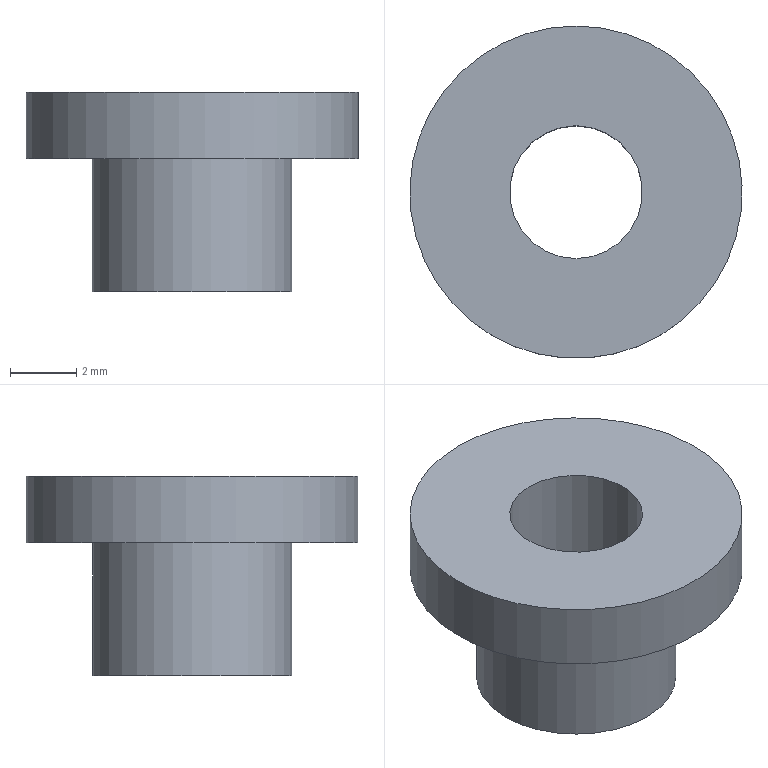Part | STEP file | 1-73.4 | 1 solid | 6 faces | box 10 x 10 x 6 mm | volume 194.779 mm3 | plane 3 | cylinder 3 | commonest cylinder face diameters 4 x1 6 x1 10 x1
STEP:
#1=CARTESIAN_POINT('',(0.,0.,0.));
#2=DIRECTION('',(0.,0.,1.));
#3=DIRECTION('',(1.,0.,0.));
#4=AXIS2_PLACEMENT_3D('',#1,#2,#3);
#5=CARTESIAN_POINT('',(0.,5.,2.));
#6=VERTEX_POINT('',#5);
#7=CARTESIAN_POINT('',(0.,0.,2.));
#8=DIRECTION('',(0.,0.,1.));
#9=DIRECTION('',(0.,1.,0.));
#10=AXIS2_PLACEMENT_3D('',#7,#8,#9);
#11=CIRCLE('',#10,5.);
#12=CARTESIAN_POINT('',(0.,-1.34,2.));
#13=DIRECTION('',(0.,0.,1.));
#14=DIRECTION('',(1.,0.,0.));
#15=AXIS2_PLACEMENT_3D('',#12,#13,#14);
#16=PLANE('',#15);
#17=CARTESIAN_POINT('',(0.,1.34));
#18=DIRECTION('',(0.,1.));
#19=AXIS2_PLACEMENT_2D('',#17,#18);
#20=CIRCLE('',#19,5.);
#21=(GEOMETRIC_REPRESENTATION_CONTEXT(2)PARAMETRIC_REPRESENTATION_CONTEXT()REPRESENTATION_CONTEXT('',''));
#22=DEFINITIONAL_REPRESENTATION('',(#20),#21);
#23=PCURVE('',#16,#22);
#24=CARTESIAN_POINT('',(0.,0.,0.));
#25=DIRECTION('',(0.,0.,1.));
#26=DIRECTION('',(0.,1.,0.));
#27=AXIS2_PLACEMENT_3D('',#24,#25,#26);
#28=CYLINDRICAL_SURFACE('',#27,5.);
#29=CARTESIAN_POINT('',(0.,2.));
#30=DIRECTION('',(1.,0.));
#31=VECTOR('',#30,1.);
#32=LINE('',#29,#31);
#33=(GEOMETRIC_REPRESENTATION_CONTEXT(2)PARAMETRIC_REPRESENTATION_CONTEXT()REPRESENTATION_CONTEXT('',''));
#34=DEFINITIONAL_REPRESENTATION('',(#32),#33);
#35=PCURVE('',#28,#34);
#36=SURFACE_CURVE('',#11,(#23,#35),.PCURVE_S1.);
#37=EDGE_CURVE('',#6,#6,#36,.T.);
#38=ORIENTED_EDGE('',*,*,#37,.T.);
#39=EDGE_LOOP('',(#38));
#40=FACE_BOUND('',#39,.T.);
#41=CARTESIAN_POINT('',(0.,2.,2.));
#42=VERTEX_POINT('',#41);
#43=CARTESIAN_POINT('',(0.,0.,2.));
#44=DIRECTION('',(0.,0.,-1.));
#45=DIRECTION('',(0.,1.,0.));
#46=AXIS2_PLACEMENT_3D('',#43,#44,#45);
#47=CIRCLE('',#46,2.);
#48=CARTESIAN_POINT('',(0.,3.34));
#49=CARTESIAN_POINT('',(3.464,3.34));
#50=CARTESIAN_POINT('',(1.732,0.3397));
#51=CARTESIAN_POINT('',(0.,-2.66));
#52=CARTESIAN_POINT('',(-1.732,0.3397));
#53=CARTESIAN_POINT('',(-3.464,3.34));
#54=CARTESIAN_POINT('',(0.,3.34));
#55=(BOUNDED_CURVE()B_SPLINE_CURVE(2,(#48,#49,#50,#51,#52,#53,#54),.UNSPECIFIED.,.T.,.F.)B_SPLINE_CURVE_WITH_KNOTS((1,2,2,2,2,1),(-2.094,0.,2.094,4.189,6.283,8.378),.UNSPECIFIED.)CURVE()GEOMETRIC_REPRESENTATION_ITEM()RATIONAL_B_SPLINE_CURVE((1.,0.5,1.,0.5,1.,0.5,1.))REPRESENTATION_ITEM(''));
#56=(GEOMETRIC_REPRESENTATION_CONTEXT(2)PARAMETRIC_REPRESENTATION_CONTEXT()REPRESENTATION_CONTEXT('',''));
#57=DEFINITIONAL_REPRESENTATION('',(#55),#56);
#58=PCURVE('',#16,#57);
#59=CARTESIAN_POINT('',(0.,0.,-4.));
#60=DIRECTION('',(0.,0.,1.));
#61=DIRECTION('',(0.,1.,0.));
#62=AXIS2_PLACEMENT_3D('',#59,#60,#61);
#63=CYLINDRICAL_SURFACE('',#62,2.);
#64=CARTESIAN_POINT('',(6.283,6.));
#65=DIRECTION('',(-1.,0.));
#66=VECTOR('',#65,1.);
#67=LINE('',#64,#66);
#68=(GEOMETRIC_REPRESENTATION_CONTEXT(2)PARAMETRIC_REPRESENTATION_CONTEXT()REPRESENTATION_CONTEXT('',''));
#69=DEFINITIONAL_REPRESENTATION('',(#67),#68);
#70=PCURVE('',#63,#69);
#71=SURFACE_CURVE('',#47,(#58,#70),.PCURVE_S1.);
#72=EDGE_CURVE('',#42,#42,#71,.T.);
#73=ORIENTED_EDGE('',*,*,#72,.T.);
#74=EDGE_LOOP('',(#73));
#75=FACE_BOUND('',#74,.T.);
#76=ADVANCED_FACE('',(#40,#75),#16,.T.);
#77=CARTESIAN_POINT('',(0.,5.,0.));
#78=VERTEX_POINT('',#77);
#79=CARTESIAN_POINT('',(0.,0.,0.));
#80=DIRECTION('',(0.,0.,1.));
#81=DIRECTION('',(0.,1.,0.));
#82=AXIS2_PLACEMENT_3D('',#79,#80,#81);
#83=CIRCLE('',#82,5.);
#84=CARTESIAN_POINT('',(0.,0.));
#85=DIRECTION('',(1.,0.));
#86=VECTOR('',#85,1.);
#87=LINE('',#84,#86);
#88=(GEOMETRIC_REPRESENTATION_CONTEXT(2)PARAMETRIC_REPRESENTATION_CONTEXT()REPRESENTATION_CONTEXT('',''));
#89=DEFINITIONAL_REPRESENTATION('',(#87),#88);
#90=PCURVE('',#28,#89);
#91=CARTESIAN_POINT('',(0.,-1.34,0.));
#92=DIRECTION('',(0.,0.,1.));
#93=DIRECTION('',(1.,0.,0.));
#94=AXIS2_PLACEMENT_3D('',#91,#92,#93);
#95=PLANE('',#94);
#96=CARTESIAN_POINT('',(0.,1.34));
#97=DIRECTION('',(0.,1.));
#98=AXIS2_PLACEMENT_2D('',#96,#97);
#99=CIRCLE('',#98,5.);
#100=(GEOMETRIC_REPRESENTATION_CONTEXT(2)PARAMETRIC_REPRESENTATION_CONTEXT()REPRESENTATION_CONTEXT('',''));
#101=DEFINITIONAL_REPRESENTATION('',(#99),#100);
#102=PCURVE('',#95,#101);
#103=SURFACE_CURVE('',#83,(#90,#102),.PCURVE_S1.);
#104=EDGE_CURVE('',#78,#78,#103,.T.);
#105=ORIENTED_EDGE('',*,*,#104,.T.);
#106=CARTESIAN_POINT('',(0.,5.,0.));
#107=DIRECTION('',(0.,0.,1.));
#108=VECTOR('',#107,1.);
#109=LINE('',#106,#108);
#110=CARTESIAN_POINT('',(6.283,0.));
#111=DIRECTION('',(0.,1.));
#112=VECTOR('',#111,1.);
#113=LINE('',#110,#112);
#114=(GEOMETRIC_REPRESENTATION_CONTEXT(2)PARAMETRIC_REPRESENTATION_CONTEXT()REPRESENTATION_CONTEXT('',''));
#115=DEFINITIONAL_REPRESENTATION('',(#113),#114);
#116=PCURVE('',#28,#115);
#117=CARTESIAN_POINT('',(0.,0.));
#118=DIRECTION('',(0.,1.));
#119=VECTOR('',#118,1.);
#120=LINE('',#117,#119);
#121=(GEOMETRIC_REPRESENTATION_CONTEXT(2)PARAMETRIC_REPRESENTATION_CONTEXT()REPRESENTATION_CONTEXT('',''));
#122=DEFINITIONAL_REPRESENTATION('',(#120),#121);
#123=PCURVE('',#28,#122);
#124=SEAM_CURVE('',#109,(#116,#123),.PCURVE_S1.);
#125=EDGE_CURVE('',#78,#6,#124,.T.);
#126=ORIENTED_EDGE('',*,*,#125,.T.);
#127=ORIENTED_EDGE('',*,*,#37,.F.);
#128=ORIENTED_EDGE('',*,*,#125,.F.);
#129=EDGE_LOOP('',(#105,#126,#127,#128));
#130=FACE_BOUND('',#129,.T.);
#131=ADVANCED_FACE('',(#130),#28,.T.);
#132=ORIENTED_EDGE('',*,*,#72,.T.);
#133=CARTESIAN_POINT('',(0.,2.,-4.));
#134=VERTEX_POINT('',#133);
#135=CARTESIAN_POINT('',(0.,2.,2.));
#136=DIRECTION('',(0.,0.,-1.));
#137=VECTOR('',#136,1.);
#138=LINE('',#135,#137);
#139=CARTESIAN_POINT('',(0.,6.));
#140=DIRECTION('',(0.,-1.));
#141=VECTOR('',#140,1.);
#142=LINE('',#139,#141);
#143=(GEOMETRIC_REPRESENTATION_CONTEXT(2)PARAMETRIC_REPRESENTATION_CONTEXT()REPRESENTATION_CONTEXT('',''));
#144=DEFINITIONAL_REPRESENTATION('',(#142),#143);
#145=PCURVE('',#63,#144);
#146=CARTESIAN_POINT('',(6.283,6.));
#147=DIRECTION('',(0.,-1.));
#148=VECTOR('',#147,1.);
#149=LINE('',#146,#148);
#150=(GEOMETRIC_REPRESENTATION_CONTEXT(2)PARAMETRIC_REPRESENTATION_CONTEXT()REPRESENTATION_CONTEXT('',''));
#151=DEFINITIONAL_REPRESENTATION('',(#149),#150);
#152=PCURVE('',#63,#151);
#153=SEAM_CURVE('',#138,(#145,#152),.PCURVE_S1.);
#154=EDGE_CURVE('',#42,#134,#153,.T.);
#155=ORIENTED_EDGE('',*,*,#154,.T.);
#156=CARTESIAN_POINT('',(0.,0.,-4.));
#157=DIRECTION('',(0.,0.,-1.));
#158=DIRECTION('',(0.,1.,0.));
#159=AXIS2_PLACEMENT_3D('',#156,#157,#158);
#160=CIRCLE('',#159,2.);
#161=CARTESIAN_POINT('',(6.283,0.));
#162=DIRECTION('',(-1.,0.));
#163=VECTOR('',#162,1.);
#164=LINE('',#161,#163);
#165=(GEOMETRIC_REPRESENTATION_CONTEXT(2)PARAMETRIC_REPRESENTATION_CONTEXT()REPRESENTATION_CONTEXT('',''));
#166=DEFINITIONAL_REPRESENTATION('',(#164),#165);
#167=PCURVE('',#63,#166);
#168=CARTESIAN_POINT('',(0.,-0.8038,-4.));
#169=DIRECTION('',(0.,0.,1.));
#170=DIRECTION('',(1.,0.,0.));
#171=AXIS2_PLACEMENT_3D('',#168,#169,#170);
#172=PLANE('',#171);
#173=CARTESIAN_POINT('',(0.,2.804));
#174=CARTESIAN_POINT('',(3.464,2.804));
#175=CARTESIAN_POINT('',(1.732,-0.1962));
#176=CARTESIAN_POINT('',(0.,-3.196));
#177=CARTESIAN_POINT('',(-1.732,-0.1962));
#178=CARTESIAN_POINT('',(-3.464,2.804));
#179=CARTESIAN_POINT('',(0.,2.804));
#180=(BOUNDED_CURVE()B_SPLINE_CURVE(2,(#173,#174,#175,#176,#177,#178,#179),.UNSPECIFIED.,.T.,.F.)B_SPLINE_CURVE_WITH_KNOTS((1,2,2,2,2,1),(-2.094,0.,2.094,4.189,6.283,8.378),.UNSPECIFIED.)CURVE()GEOMETRIC_REPRESENTATION_ITEM()RATIONAL_B_SPLINE_CURVE((1.,0.5,1.,0.5,1.,0.5,1.))REPRESENTATION_ITEM(''));
#181=(GEOMETRIC_REPRESENTATION_CONTEXT(2)PARAMETRIC_REPRESENTATION_CONTEXT()REPRESENTATION_CONTEXT('',''));
#182=DEFINITIONAL_REPRESENTATION('',(#180),#181);
#183=PCURVE('',#172,#182);
#184=SURFACE_CURVE('',#160,(#167,#183),.PCURVE_S1.);
#185=EDGE_CURVE('',#134,#134,#184,.T.);
#186=ORIENTED_EDGE('',*,*,#185,.F.);
#187=ORIENTED_EDGE('',*,*,#154,.F.);
#188=EDGE_LOOP('',(#132,#155,#186,#187));
#189=FACE_BOUND('',#188,.F.);
#190=ADVANCED_FACE('',(#189),#63,.F.);
#191=ORIENTED_EDGE('',*,*,#104,.T.);
#192=EDGE_LOOP('',(#191));
#193=FACE_BOUND('',#192,.F.);
#194=CARTESIAN_POINT('',(0.,3.,0.));
#195=VERTEX_POINT('',#194);
#196=CARTESIAN_POINT('',(0.,0.,0.));
#197=DIRECTION('',(0.,0.,1.));
#198=DIRECTION('',(0.,1.,0.));
#199=AXIS2_PLACEMENT_3D('',#196,#197,#198);
#200=CIRCLE('',#199,3.);
#201=CARTESIAN_POINT('',(0.,1.34));
#202=DIRECTION('',(0.,1.));
#203=AXIS2_PLACEMENT_2D('',#201,#202);
#204=CIRCLE('',#203,3.);
#205=(GEOMETRIC_REPRESENTATION_CONTEXT(2)PARAMETRIC_REPRESENTATION_CONTEXT()REPRESENTATION_CONTEXT('',''));
#206=DEFINITIONAL_REPRESENTATION('',(#204),#205);
#207=PCURVE('',#95,#206);
#208=CARTESIAN_POINT('',(0.,0.,0.));
#209=DIRECTION('',(0.,0.,-1.));
#210=DIRECTION('',(0.,1.,0.));
#211=AXIS2_PLACEMENT_3D('',#208,#209,#210);
#212=CYLINDRICAL_SURFACE('',#211,3.);
#213=CARTESIAN_POINT('',(6.283,0.));
#214=DIRECTION('',(-1.,0.));
#215=VECTOR('',#214,1.);
#216=LINE('',#213,#215);
#217=(GEOMETRIC_REPRESENTATION_CONTEXT(2)PARAMETRIC_REPRESENTATION_CONTEXT()REPRESENTATION_CONTEXT('',''));
#218=DEFINITIONAL_REPRESENTATION('',(#216),#217);
#219=PCURVE('',#212,#218);
#220=SURFACE_CURVE('',#200,(#207,#219),.PCURVE_S1.);
#221=EDGE_CURVE('',#195,#195,#220,.T.);
#222=ORIENTED_EDGE('',*,*,#221,.F.);
#223=EDGE_LOOP('',(#222));
#224=FACE_BOUND('',#223,.F.);
#225=ADVANCED_FACE('',(#193,#224),#95,.F.);
#226=CARTESIAN_POINT('',(0.,3.,-4.));
#227=VERTEX_POINT('',#226);
#228=CARTESIAN_POINT('',(0.,3.,0.));
#229=DIRECTION('',(0.,0.,-1.));
#230=VECTOR('',#229,1.);
#231=LINE('',#228,#230);
#232=CARTESIAN_POINT('',(6.283,0.));
#233=DIRECTION('',(0.,1.));
#234=VECTOR('',#233,1.);
#235=LINE('',#232,#234);
#236=(GEOMETRIC_REPRESENTATION_CONTEXT(2)PARAMETRIC_REPRESENTATION_CONTEXT()REPRESENTATION_CONTEXT('',''));
#237=DEFINITIONAL_REPRESENTATION('',(#235),#236);
#238=PCURVE('',#212,#237);
#239=CARTESIAN_POINT('',(0.,0.));
#240=DIRECTION('',(0.,1.));
#241=VECTOR('',#240,1.);
#242=LINE('',#239,#241);
#243=(GEOMETRIC_REPRESENTATION_CONTEXT(2)PARAMETRIC_REPRESENTATION_CONTEXT()REPRESENTATION_CONTEXT('',''));
#244=DEFINITIONAL_REPRESENTATION('',(#242),#243);
#245=PCURVE('',#212,#244);
#246=SEAM_CURVE('',#231,(#238,#245),.PCURVE_S1.);
#247=EDGE_CURVE('',#195,#227,#246,.T.);
#248=ORIENTED_EDGE('',*,*,#247,.T.);
#249=CARTESIAN_POINT('',(0.,0.,-4.));
#250=DIRECTION('',(0.,0.,1.));
#251=DIRECTION('',(0.,1.,0.));
#252=AXIS2_PLACEMENT_3D('',#249,#250,#251);
#253=CIRCLE('',#252,3.);
#254=CARTESIAN_POINT('',(6.283,4.));
#255=DIRECTION('',(-1.,0.));
#256=VECTOR('',#255,1.);
#257=LINE('',#254,#256);
#258=(GEOMETRIC_REPRESENTATION_CONTEXT(2)PARAMETRIC_REPRESENTATION_CONTEXT()REPRESENTATION_CONTEXT('',''));
#259=DEFINITIONAL_REPRESENTATION('',(#257),#258);
#260=PCURVE('',#212,#259);
#261=CARTESIAN_POINT('',(0.,0.8038));
#262=DIRECTION('',(0.,1.));
#263=AXIS2_PLACEMENT_2D('',#261,#262);
#264=CIRCLE('',#263,3.);
#265=(GEOMETRIC_REPRESENTATION_CONTEXT(2)PARAMETRIC_REPRESENTATION_CONTEXT()REPRESENTATION_CONTEXT('',''));
#266=DEFINITIONAL_REPRESENTATION('',(#264),#265);
#267=PCURVE('',#172,#266);
#268=SURFACE_CURVE('',#253,(#260,#267),.PCURVE_S1.);
#269=EDGE_CURVE('',#227,#227,#268,.T.);
#270=ORIENTED_EDGE('',*,*,#269,.T.);
#271=ORIENTED_EDGE('',*,*,#247,.F.);
#272=ORIENTED_EDGE('',*,*,#221,.F.);
#273=EDGE_LOOP('',(#248,#270,#271,#272));
#274=FACE_BOUND('',#273,.T.);
#275=ADVANCED_FACE('',(#274),#212,.T.);
#276=ORIENTED_EDGE('',*,*,#269,.T.);
#277=EDGE_LOOP('',(#276));
#278=FACE_BOUND('',#277,.F.);
#279=ORIENTED_EDGE('',*,*,#185,.T.);
#280=EDGE_LOOP('',(#279));
#281=FACE_BOUND('',#280,.F.);
#282=ADVANCED_FACE('',(#278,#281),#172,.F.);
#283=CLOSED_SHELL('',(#76,#131,#190,#225,#275,#282));
#284=MANIFOLD_SOLID_BREP('',#283);
#285=(LENGTH_UNIT()NAMED_UNIT(*)SI_UNIT(.MILLI.,.METRE.));
#286=UNCERTAINTY_MEASURE_WITH_UNIT(LENGTH_MEASURE(0.0000001),#285,'','');
#287=(NAMED_UNIT(*)PLANE_ANGLE_UNIT()SI_UNIT($,.RADIAN.));
#288=(NAMED_UNIT(*)SI_UNIT($,.STERADIAN.)SOLID_ANGLE_UNIT());
#289=(GEOMETRIC_REPRESENTATION_CONTEXT(3)GLOBAL_UNCERTAINTY_ASSIGNED_CONTEXT((#286))GLOBAL_UNIT_ASSIGNED_CONTEXT((#285,#287,#288))REPRESENTATION_CONTEXT('',''));
#290=ADVANCED_BREP_SHAPE_REPRESENTATION('',(#4,#284),#289);